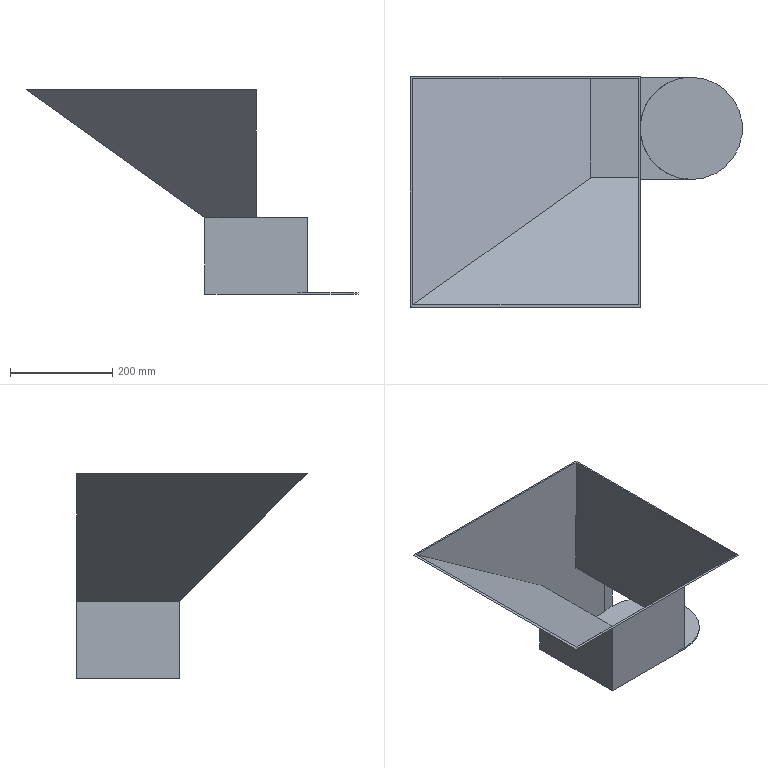Part | SolidWorks | features ICE 2, Blend 1, Extrusion 1, Shell 1 | 1 solid | 20 faces | box 650 x 450 x 400 mm | volume 1573727 mm3 | plane 18 | cylinder 2 | commonest cylinder face diameters 200 x2
STEP:
#1=CARTESIAN_POINT('',(100.,-100.,3.));
#2=VERTEX_POINT('',#1);
#3=CARTESIAN_POINT('',(75.69,-97.,3.));
#4=VERTEX_POINT('',#3);
#5=CARTESIAN_POINT('',(100.,0.,3.));
#6=DIRECTION('',(0.,0.,-1.));
#7=DIRECTION('',(-1.,0.,0.));
#8=AXIS2_PLACEMENT_3D('',#5,#6,#7);
#9=CIRCLE('',#8,100.);
#10=EDGE_CURVE('',#2,#4,#9,.T.);
#11=ORIENTED_EDGE('',*,*,#10,.T.);
#12=CARTESIAN_POINT('',(75.69,-97.,147.));
#13=VERTEX_POINT('',#12);
#14=CARTESIAN_POINT('',(75.69,-97.,-50.));
#15=DIRECTION('',(0.,0.,-1.));
#16=VECTOR('',#15,1000.);
#17=LINE('',#14,#16);
#18=EDGE_CURVE('',#13,#4,#17,.T.);
#19=ORIENTED_EDGE('',*,*,#18,.F.);
#20=CARTESIAN_POINT('',(75.69,97.,147.));
#21=VERTEX_POINT('',#20);
#22=CARTESIAN_POINT('',(100.,0.,147.));
#23=DIRECTION('',(0.,0.,1.));
#24=DIRECTION('',(-1.,0.,0.));
#25=AXIS2_PLACEMENT_3D('',#22,#23,#24);
#26=CIRCLE('',#25,100.);
#27=EDGE_CURVE('',#21,#13,#26,.T.);
#28=ORIENTED_EDGE('',*,*,#27,.F.);
#29=CARTESIAN_POINT('',(75.69,97.,3.));
#30=VERTEX_POINT('',#29);
#31=CARTESIAN_POINT('',(75.69,97.,75.));
#32=DIRECTION('',(0.,0.,-1.));
#33=VECTOR('',#32,1000.);
#34=LINE('',#31,#33);
#35=EDGE_CURVE('',#21,#30,#34,.T.);
#36=ORIENTED_EDGE('',*,*,#35,.T.);
#37=CARTESIAN_POINT('',(100.,100.,3.));
#38=VERTEX_POINT('',#37);
#39=CARTESIAN_POINT('',(100.,0.,3.));
#40=DIRECTION('',(0.,0.,-1.));
#41=DIRECTION('',(-1.,0.,0.));
#42=AXIS2_PLACEMENT_3D('',#39,#40,#41);
#43=CIRCLE('',#42,100.);
#44=EDGE_CURVE('',#30,#38,#43,.T.);
#45=ORIENTED_EDGE('',*,*,#44,.T.);
#46=CARTESIAN_POINT('',(100.,100.,150.));
#47=VERTEX_POINT('',#46);
#48=CARTESIAN_POINT('',(100.,100.,150.));
#49=DIRECTION('',(0.,0.,-1.));
#50=VECTOR('',#49,1000.);
#51=LINE('',#48,#50);
#52=EDGE_CURVE('',#47,#38,#51,.T.);
#53=ORIENTED_EDGE('',*,*,#52,.F.);
#54=CARTESIAN_POINT('',(0.,0.,150.));
#55=VERTEX_POINT('',#54);
#56=CARTESIAN_POINT('',(100.,0.,150.));
#57=DIRECTION('',(0.,0.,1.));
#58=DIRECTION('',(1.,0.,0.));
#59=AXIS2_PLACEMENT_3D('',#56,#57,#58);
#60=CIRCLE('',#59,100.);
#61=EDGE_CURVE('',#47,#55,#60,.T.);
#62=ORIENTED_EDGE('',*,*,#61,.T.);
#63=CARTESIAN_POINT('',(100.,-100.,150.));
#64=VERTEX_POINT('',#63);
#65=CARTESIAN_POINT('',(100.,0.,150.));
#66=DIRECTION('',(0.,0.,1.));
#67=DIRECTION('',(1.,0.,0.));
#68=AXIS2_PLACEMENT_3D('',#65,#66,#67);
#69=CIRCLE('',#68,100.);
#70=EDGE_CURVE('',#55,#64,#69,.T.);
#71=ORIENTED_EDGE('',*,*,#70,.T.);
#72=CARTESIAN_POINT('',(100.,-100.,150.));
#73=DIRECTION('',(0.,0.,-1.));
#74=VECTOR('',#73,1000.);
#75=LINE('',#72,#74);
#76=EDGE_CURVE('',#64,#2,#75,.T.);
#77=ORIENTED_EDGE('',*,*,#76,.T.);
#78=EDGE_LOOP('',(#11,#19,#28,#36,#45,#53,#62,#71,#77));
#79=FACE_OUTER_BOUND('',#78,.T.);
#80=CARTESIAN_POINT('',(100.,0.,-50.));
#81=DIRECTION('',(0.,0.,1.));
#82=DIRECTION('',(1.,0.,0.));
#83=AXIS2_PLACEMENT_3D('',#80,#81,#82);
#84=CYLINDRICAL_SURFACE('',#83,100.);
#85=ADVANCED_FACE('',(#79),#84,.F.);
#86=CARTESIAN_POINT('',(-97.,-97.,151.243));
#87=VERTEX_POINT('',#86);
#88=CARTESIAN_POINT('',(-97.,-97.,3.));
#89=VERTEX_POINT('',#88);
#90=CARTESIAN_POINT('',(-97.,-97.,150.));
#91=DIRECTION('',(0.,0.,-1.));
#92=VECTOR('',#91,1000.);
#93=LINE('',#90,#92);
#94=EDGE_CURVE('',#87,#89,#93,.T.);
#95=ORIENTED_EDGE('',*,*,#94,.T.);
#96=CARTESIAN_POINT('',(-97.,97.,3.));
#97=VERTEX_POINT('',#96);
#98=CARTESIAN_POINT('',(-97.,0.,3.));
#99=DIRECTION('',(0.,-1.,0.));
#100=VECTOR('',#99,1000.);
#101=LINE('',#98,#100);
#102=EDGE_CURVE('',#97,#89,#101,.T.);
#103=ORIENTED_EDGE('',*,*,#102,.F.);
#104=CARTESIAN_POINT('',(-97.,97.,151.544));
#105=VERTEX_POINT('',#104);
#106=CARTESIAN_POINT('',(-97.,97.,150.));
#107=DIRECTION('',(0.,0.,-1.));
#108=VECTOR('',#107,1000.);
#109=LINE('',#106,#108);
#110=EDGE_CURVE('',#105,#97,#109,.T.);
#111=ORIENTED_EDGE('',*,*,#110,.F.);
#112=CARTESIAN_POINT('',(-97.,-97.301,151.544));
#113=VERTEX_POINT('',#112);
#114=CARTESIAN_POINT('',(-97.,0.,151.544));
#115=DIRECTION('',(0.,-1.,0.));
#116=VECTOR('',#115,1000.);
#117=LINE('',#114,#116);
#118=EDGE_CURVE('',#105,#113,#117,.T.);
#119=ORIENTED_EDGE('',*,*,#118,.T.);
#120=CARTESIAN_POINT('',(-97.,27.121,27.121));
#121=DIRECTION('',(0.,-0.7071,0.7071));
#122=VECTOR('',#121,1000.);
#123=LINE('',#120,#122);
#124=EDGE_CURVE('',#87,#113,#123,.T.);
#125=ORIENTED_EDGE('',*,*,#124,.F.);
#126=EDGE_LOOP('',(#95,#103,#111,#119,#125));
#127=FACE_OUTER_BOUND('',#126,.T.);
#128=CARTESIAN_POINT('',(-97.,100.,150.));
#129=DIRECTION('',(1.,0.,0.));
#130=DIRECTION('',(0.,1.,0.));
#131=AXIS2_PLACEMENT_3D('',#128,#129,#130);
#132=PLANE('',#131);
#133=ADVANCED_FACE('',(#127),#132,.T.);
#134=ORIENTED_EDGE('',*,*,#18,.T.);
#135=CARTESIAN_POINT('',(0.,-97.,3.));
#136=DIRECTION('',(1.,0.,0.));
#137=VECTOR('',#136,1000.);
#138=LINE('',#135,#137);
#139=EDGE_CURVE('',#89,#4,#138,.T.);
#140=ORIENTED_EDGE('',*,*,#139,.F.);
#141=ORIENTED_EDGE('',*,*,#94,.F.);
#142=CARTESIAN_POINT('',(-3.,-97.,151.243));
#143=VERTEX_POINT('',#142);
#144=CARTESIAN_POINT('',(0.,-97.,151.243));
#145=DIRECTION('',(1.,0.,0.));
#146=VECTOR('',#145,1000.);
#147=LINE('',#144,#146);
#148=EDGE_CURVE('',#87,#143,#147,.T.);
#149=ORIENTED_EDGE('',*,*,#148,.T.);
#150=CARTESIAN_POINT('',(-3.,-97.,147.));
#151=VERTEX_POINT('',#150);
#152=CARTESIAN_POINT('',(-3.,-97.,150.));
#153=DIRECTION('',(0.,0.,-1.));
#154=VECTOR('',#153,1000.);
#155=LINE('',#152,#154);
#156=EDGE_CURVE('',#143,#151,#155,.T.);
#157=ORIENTED_EDGE('',*,*,#156,.T.);
#158=CARTESIAN_POINT('',(0.,-97.,147.));
#159=DIRECTION('',(1.,0.,0.));
#160=VECTOR('',#159,1000.);
#161=LINE('',#158,#160);
#162=EDGE_CURVE('',#151,#13,#161,.T.);
#163=ORIENTED_EDGE('',*,*,#162,.T.);
#164=EDGE_LOOP('',(#134,#140,#141,#149,#157,#163));
#165=FACE_OUTER_BOUND('',#164,.T.);
#166=CARTESIAN_POINT('',(100.,-97.,150.));
#167=DIRECTION('',(0.,1.,0.));
#168=DIRECTION('',(-1.,0.,0.));
#169=AXIS2_PLACEMENT_3D('',#166,#167,#168);
#170=PLANE('',#169);
#171=ADVANCED_FACE('',(#165),#170,.T.);
#172=ORIENTED_EDGE('',*,*,#110,.T.);
#173=CARTESIAN_POINT('',(0.,97.,3.));
#174=DIRECTION('',(-1.,0.,0.));
#175=VECTOR('',#174,1000.);
#176=LINE('',#173,#175);
#177=EDGE_CURVE('',#30,#97,#176,.T.);
#178=ORIENTED_EDGE('',*,*,#177,.F.);
#179=ORIENTED_EDGE('',*,*,#35,.F.);
#180=CARTESIAN_POINT('',(-3.,97.,147.));
#181=VERTEX_POINT('',#180);
#182=CARTESIAN_POINT('',(0.,97.,147.));
#183=DIRECTION('',(-1.,0.,0.));
#184=VECTOR('',#183,1000.);
#185=LINE('',#182,#184);
#186=EDGE_CURVE('',#21,#181,#185,.T.);
#187=ORIENTED_EDGE('',*,*,#186,.T.);
#188=CARTESIAN_POINT('',(-3.,97.,400.));
#189=VERTEX_POINT('',#188);
#190=CARTESIAN_POINT('',(-3.,97.,0.));
#191=DIRECTION('',(0.,0.,-1.));
#192=VECTOR('',#191,1000.);
#193=LINE('',#190,#192);
#194=EDGE_CURVE('',#189,#181,#193,.T.);
#195=ORIENTED_EDGE('',*,*,#194,.F.);
#196=CARTESIAN_POINT('',(-444.839,97.,400.));
#197=VERTEX_POINT('',#196);
#198=CARTESIAN_POINT('',(0.,97.,400.));
#199=DIRECTION('',(-1.,0.,0.));
#200=VECTOR('',#199,1000.);
#201=LINE('',#198,#200);
#202=EDGE_CURVE('',#189,#197,#201,.T.);
#203=ORIENTED_EDGE('',*,*,#202,.T.);
#204=CARTESIAN_POINT('',(34.176,97.,57.847));
#205=DIRECTION('',(0.8137,0.,-0.5812));
#206=VECTOR('',#205,1000.);
#207=LINE('',#204,#206);
#208=EDGE_CURVE('',#197,#105,#207,.T.);
#209=ORIENTED_EDGE('',*,*,#208,.T.);
#210=EDGE_LOOP('',(#172,#178,#179,#187,#195,#203,#209));
#211=FACE_OUTER_BOUND('',#210,.T.);
#212=CARTESIAN_POINT('',(100.,97.,150.));
#213=DIRECTION('',(0.,-1.,0.));
#214=DIRECTION('',(1.,0.,0.));
#215=AXIS2_PLACEMENT_3D('',#212,#213,#214);
#216=PLANE('',#215);
#217=ADVANCED_FACE('',(#211),#216,.T.);
#218=CARTESIAN_POINT('',(100.,100.,0.));
#219=VERTEX_POINT('',#218);
#220=CARTESIAN_POINT('',(-100.,100.,0.));
#221=VERTEX_POINT('',#220);
#222=CARTESIAN_POINT('',(100.,100.,0.));
#223=DIRECTION('',(-1.,0.,0.));
#224=VECTOR('',#223,1000.);
#225=LINE('',#222,#224);
#226=EDGE_CURVE('',#219,#221,#225,.T.);
#227=ORIENTED_EDGE('',*,*,#226,.F.);
#228=CARTESIAN_POINT('',(100.,-100.,0.));
#229=VERTEX_POINT('',#228);
#230=CARTESIAN_POINT('',(100.,0.,0.));
#231=DIRECTION('',(0.,0.,-1.));
#232=DIRECTION('',(-1.,0.,0.));
#233=AXIS2_PLACEMENT_3D('',#230,#231,#232);
#234=CIRCLE('',#233,100.);
#235=EDGE_CURVE('',#219,#229,#234,.T.);
#236=ORIENTED_EDGE('',*,*,#235,.T.);
#237=CARTESIAN_POINT('',(-100.,-100.,0.));
#238=VERTEX_POINT('',#237);
#239=CARTESIAN_POINT('',(100.,-100.,0.));
#240=DIRECTION('',(1.,0.,0.));
#241=VECTOR('',#240,1000.);
#242=LINE('',#239,#241);
#243=EDGE_CURVE('',#238,#229,#242,.T.);
#244=ORIENTED_EDGE('',*,*,#243,.F.);
#245=CARTESIAN_POINT('',(-100.,100.,0.));
#246=DIRECTION('',(0.,-1.,0.));
#247=VECTOR('',#246,1000.);
#248=LINE('',#245,#247);
#249=EDGE_CURVE('',#221,#238,#248,.T.);
#250=ORIENTED_EDGE('',*,*,#249,.F.);
#251=EDGE_LOOP('',(#227,#236,#244,#250));
#252=FACE_OUTER_BOUND('',#251,.T.);
#253=CARTESIAN_POINT('',(0.,0.,0.));
#254=DIRECTION('',(0.,0.,-1.));
#255=DIRECTION('',(-1.,0.,0.));
#256=AXIS2_PLACEMENT_3D('',#253,#254,#255);
#257=PLANE('',#256);
#258=ADVANCED_FACE('',(#252),#257,.T.);
#259=CARTESIAN_POINT('',(0.,-350.,400.));
#260=VERTEX_POINT('',#259);
#261=CARTESIAN_POINT('',(0.,100.,400.));
#262=VERTEX_POINT('',#261);
#263=CARTESIAN_POINT('',(0.,100.,400.));
#264=DIRECTION('',(0.,1.,0.));
#265=VECTOR('',#264,1000.);
#266=LINE('',#263,#265);
#267=EDGE_CURVE('',#260,#262,#266,.T.);
#268=ORIENTED_EDGE('',*,*,#267,.T.);
#269=CARTESIAN_POINT('',(-450.,100.,400.));
#270=VERTEX_POINT('',#269);
#271=CARTESIAN_POINT('',(0.,100.,400.));
#272=DIRECTION('',(-1.,0.,0.));
#273=VECTOR('',#272,1000.);
#274=LINE('',#271,#273);
#275=EDGE_CURVE('',#262,#270,#274,.T.);
#276=ORIENTED_EDGE('',*,*,#275,.T.);
#277=CARTESIAN_POINT('',(-450.,-350.,400.));
#278=VERTEX_POINT('',#277);
#279=CARTESIAN_POINT('',(-450.,100.,400.));
#280=DIRECTION('',(0.,-1.,0.));
#281=VECTOR('',#280,1000.);
#282=LINE('',#279,#281);
#283=EDGE_CURVE('',#270,#278,#282,.T.);
#284=ORIENTED_EDGE('',*,*,#283,.T.);
#285=CARTESIAN_POINT('',(0.,-350.,400.));
#286=DIRECTION('',(1.,0.,0.));
#287=VECTOR('',#286,1000.);
#288=LINE('',#285,#287);
#289=EDGE_CURVE('',#278,#260,#288,.T.);
#290=ORIENTED_EDGE('',*,*,#289,.T.);
#291=EDGE_LOOP('',(#268,#276,#284,#290));
#292=FACE_OUTER_BOUND('',#291,.T.);
#293=CARTESIAN_POINT('',(-3.,-345.757,400.));
#294=VERTEX_POINT('',#293);
#295=CARTESIAN_POINT('',(-3.,0.,400.));
#296=DIRECTION('',(0.,1.,0.));
#297=VECTOR('',#296,1000.);
#298=LINE('',#295,#297);
#299=EDGE_CURVE('',#294,#189,#298,.T.);
#300=ORIENTED_EDGE('',*,*,#299,.F.);
#301=CARTESIAN_POINT('',(-444.839,-345.757,400.));
#302=VERTEX_POINT('',#301);
#303=CARTESIAN_POINT('',(0.,-345.757,400.));
#304=DIRECTION('',(1.,0.,0.));
#305=VECTOR('',#304,1000.);
#306=LINE('',#303,#305);
#307=EDGE_CURVE('',#302,#294,#306,.T.);
#308=ORIENTED_EDGE('',*,*,#307,.F.);
#309=CARTESIAN_POINT('',(-444.839,0.,400.));
#310=DIRECTION('',(0.,-1.,0.));
#311=VECTOR('',#310,1000.);
#312=LINE('',#309,#311);
#313=EDGE_CURVE('',#197,#302,#312,.T.);
#314=ORIENTED_EDGE('',*,*,#313,.F.);
#315=ORIENTED_EDGE('',*,*,#202,.F.);
#316=EDGE_LOOP('',(#300,#308,#314,#315));
#317=FACE_BOUND('',#316,.T.);
#318=CARTESIAN_POINT('',(0.,0.,400.));
#319=DIRECTION('',(0.,0.,-1.));
#320=DIRECTION('',(-1.,0.,0.));
#321=AXIS2_PLACEMENT_3D('',#318,#319,#320);
#322=PLANE('',#321);
#323=ADVANCED_FACE('',(#292,#317),#322,.F.);
#324=CARTESIAN_POINT('',(0.,100.,150.));
#325=VERTEX_POINT('',#324);
#326=CARTESIAN_POINT('',(0.,100.,150.));
#327=DIRECTION('',(0.,1.,0.));
#328=VECTOR('',#327,1000.);
#329=LINE('',#326,#328);
#330=EDGE_CURVE('',#55,#325,#329,.T.);
#331=ORIENTED_EDGE('',*,*,#330,.F.);
#332=ORIENTED_EDGE('',*,*,#61,.F.);
#333=CARTESIAN_POINT('',(100.,100.,150.));
#334=DIRECTION('',(-1.,0.,0.));
#335=VECTOR('',#334,1000.);
#336=LINE('',#333,#335);
#337=EDGE_CURVE('',#47,#325,#336,.T.);
#338=ORIENTED_EDGE('',*,*,#337,.T.);
#339=EDGE_LOOP('',(#331,#332,#338));
#340=FACE_OUTER_BOUND('',#339,.T.);
#341=CARTESIAN_POINT('',(0.,0.,150.));
#342=DIRECTION('',(0.,0.,-1.));
#343=DIRECTION('',(-1.,0.,0.));
#344=AXIS2_PLACEMENT_3D('',#341,#342,#343);
#345=PLANE('',#344);
#346=ADVANCED_FACE('',(#340),#345,.F.);
#347=ORIENTED_EDGE('',*,*,#249,.T.);
#348=CARTESIAN_POINT('',(-100.,-100.,150.));
#349=VERTEX_POINT('',#348);
#350=CARTESIAN_POINT('',(-100.,-100.,150.));
#351=DIRECTION('',(0.,0.,-1.));
#352=VECTOR('',#351,1000.);
#353=LINE('',#350,#352);
#354=EDGE_CURVE('',#349,#238,#353,.T.);
#355=ORIENTED_EDGE('',*,*,#354,.F.);
#356=CARTESIAN_POINT('',(-100.,100.,150.));
#357=VERTEX_POINT('',#356);
#358=CARTESIAN_POINT('',(-100.,0.,150.));
#359=DIRECTION('',(0.,-1.,0.));
#360=VECTOR('',#359,1000.);
#361=LINE('',#358,#360);
#362=EDGE_CURVE('',#357,#349,#361,.T.);
#363=ORIENTED_EDGE('',*,*,#362,.F.);
#364=CARTESIAN_POINT('',(-100.,100.,150.));
#365=DIRECTION('',(0.,0.,-1.));
#366=VECTOR('',#365,1000.);
#367=LINE('',#364,#366);
#368=EDGE_CURVE('',#357,#221,#367,.T.);
#369=ORIENTED_EDGE('',*,*,#368,.T.);
#370=EDGE_LOOP('',(#347,#355,#363,#369));
#371=FACE_OUTER_BOUND('',#370,.T.);
#372=CARTESIAN_POINT('',(-100.,100.,150.));
#373=DIRECTION('',(1.,0.,0.));
#374=DIRECTION('',(0.,1.,0.));
#375=AXIS2_PLACEMENT_3D('',#372,#373,#374);
#376=PLANE('',#375);
#377=ADVANCED_FACE('',(#371),#376,.F.);
#378=ORIENTED_EDGE('',*,*,#243,.T.);
#379=CARTESIAN_POINT('',(100.,-100.,3.));
#380=DIRECTION('',(0.,0.,-1.));
#381=VECTOR('',#380,1000.);
#382=LINE('',#379,#381);
#383=EDGE_CURVE('',#2,#229,#382,.T.);
#384=ORIENTED_EDGE('',*,*,#383,.F.);
#385=ORIENTED_EDGE('',*,*,#76,.F.);
#386=CARTESIAN_POINT('',(0.,-100.,150.));
#387=VERTEX_POINT('',#386);
#388=CARTESIAN_POINT('',(100.,-100.,150.));
#389=DIRECTION('',(1.,0.,0.));
#390=VECTOR('',#389,1000.);
#391=LINE('',#388,#390);
#392=EDGE_CURVE('',#387,#64,#391,.T.);
#393=ORIENTED_EDGE('',*,*,#392,.F.);
#394=CARTESIAN_POINT('',(0.,-100.,150.));
#395=DIRECTION('',(1.,0.,0.));
#396=VECTOR('',#395,1000.);
#397=LINE('',#394,#396);
#398=EDGE_CURVE('',#349,#387,#397,.T.);
#399=ORIENTED_EDGE('',*,*,#398,.F.);
#400=ORIENTED_EDGE('',*,*,#354,.T.);
#401=EDGE_LOOP('',(#378,#384,#385,#393,#399,#400));
#402=FACE_OUTER_BOUND('',#401,.T.);
#403=CARTESIAN_POINT('',(100.,-100.,150.));
#404=DIRECTION('',(0.,1.,0.));
#405=DIRECTION('',(-1.,0.,0.));
#406=AXIS2_PLACEMENT_3D('',#403,#404,#405);
#407=PLANE('',#406);
#408=ADVANCED_FACE('',(#402),#407,.F.);
#409=ORIENTED_EDGE('',*,*,#226,.T.);
#410=ORIENTED_EDGE('',*,*,#368,.F.);
#411=CARTESIAN_POINT('',(-450.,100.,400.));
#412=DIRECTION('',(0.8137,0.,-0.5812));
#413=VECTOR('',#412,1000.);
#414=LINE('',#411,#413);
#415=EDGE_CURVE('',#270,#357,#414,.T.);
#416=ORIENTED_EDGE('',*,*,#415,.F.);
#417=ORIENTED_EDGE('',*,*,#275,.F.);
#418=CARTESIAN_POINT('',(0.,100.,400.));
#419=DIRECTION('',(0.,0.,-1.));
#420=VECTOR('',#419,1000.);
#421=LINE('',#418,#420);
#422=EDGE_CURVE('',#262,#325,#421,.T.);
#423=ORIENTED_EDGE('',*,*,#422,.T.);
#424=ORIENTED_EDGE('',*,*,#337,.F.);
#425=ORIENTED_EDGE('',*,*,#52,.T.);
#426=CARTESIAN_POINT('',(100.,100.,3.));
#427=DIRECTION('',(0.,0.,-1.));
#428=VECTOR('',#427,1000.);
#429=LINE('',#426,#428);
#430=EDGE_CURVE('',#38,#219,#429,.T.);
#431=ORIENTED_EDGE('',*,*,#430,.T.);
#432=EDGE_LOOP('',(#409,#410,#416,#417,#423,#424,#425,#431));
#433=FACE_OUTER_BOUND('',#432,.T.);
#434=CARTESIAN_POINT('',(100.,100.,150.));
#435=DIRECTION('',(0.,-1.,0.));
#436=DIRECTION('',(1.,0.,0.));
#437=AXIS2_PLACEMENT_3D('',#434,#435,#436);
#438=PLANE('',#437);
#439=ADVANCED_FACE('',(#433),#438,.F.);
#440=ORIENTED_EDGE('',*,*,#392,.T.);
#441=ORIENTED_EDGE('',*,*,#70,.F.);
#442=CARTESIAN_POINT('',(0.,100.,150.));
#443=DIRECTION('',(0.,1.,0.));
#444=VECTOR('',#443,1000.);
#445=LINE('',#442,#444);
#446=EDGE_CURVE('',#387,#55,#445,.T.);
#447=ORIENTED_EDGE('',*,*,#446,.F.);
#448=EDGE_LOOP('',(#440,#441,#447));
#449=FACE_OUTER_BOUND('',#448,.T.);
#450=CARTESIAN_POINT('',(0.,0.,150.));
#451=DIRECTION('',(0.,0.,-1.));
#452=DIRECTION('',(-1.,0.,0.));
#453=AXIS2_PLACEMENT_3D('',#450,#451,#452);
#454=PLANE('',#453);
#455=ADVANCED_FACE('',(#449),#454,.F.);
#456=CARTESIAN_POINT('',(0.,-350.,400.));
#457=DIRECTION('',(0.,0.7071,-0.7071));
#458=VECTOR('',#457,1000.);
#459=LINE('',#456,#458);
#460=EDGE_CURVE('',#260,#387,#459,.T.);
#461=ORIENTED_EDGE('',*,*,#460,.T.);
#462=ORIENTED_EDGE('',*,*,#446,.T.);
#463=ORIENTED_EDGE('',*,*,#330,.T.);
#464=ORIENTED_EDGE('',*,*,#422,.F.);
#465=ORIENTED_EDGE('',*,*,#267,.F.);
#466=EDGE_LOOP('',(#461,#462,#463,#464,#465));
#467=FACE_OUTER_BOUND('',#466,.T.);
#468=CARTESIAN_POINT('',(0.,0.,0.));
#469=DIRECTION('',(1.,0.,0.));
#470=DIRECTION('',(0.,0.,-1.));
#471=AXIS2_PLACEMENT_3D('',#468,#469,#470);
#472=PLANE('',#471);
#473=ADVANCED_FACE('',(#467),#472,.T.);
#474=CARTESIAN_POINT('',(-450.,-350.,400.));
#475=DIRECTION('',(0.7035,0.5025,-0.5025));
#476=VECTOR('',#475,1000.);
#477=LINE('',#474,#476);
#478=EDGE_CURVE('',#278,#349,#477,.T.);
#479=ORIENTED_EDGE('',*,*,#478,.T.);
#480=ORIENTED_EDGE('',*,*,#398,.T.);
#481=ORIENTED_EDGE('',*,*,#460,.F.);
#482=ORIENTED_EDGE('',*,*,#289,.F.);
#483=EDGE_LOOP('',(#479,#480,#481,#482));
#484=FACE_OUTER_BOUND('',#483,.T.);
#485=CARTESIAN_POINT('',(0.,25.,25.));
#486=DIRECTION('',(0.,-0.7071,-0.7071));
#487=DIRECTION('',(0.,0.7071,-0.7071));
#488=AXIS2_PLACEMENT_3D('',#485,#486,#487);
#489=PLANE('',#488);
#490=ADVANCED_FACE('',(#484),#489,.T.);
#491=ORIENTED_EDGE('',*,*,#415,.T.);
#492=ORIENTED_EDGE('',*,*,#362,.T.);
#493=ORIENTED_EDGE('',*,*,#478,.F.);
#494=ORIENTED_EDGE('',*,*,#283,.F.);
#495=EDGE_LOOP('',(#491,#492,#493,#494));
#496=FACE_OUTER_BOUND('',#495,.T.);
#497=CARTESIAN_POINT('',(37.162,0.,52.027));
#498=DIRECTION('',(-0.5812,0.,-0.8137));
#499=DIRECTION('',(-0.8137,0.,0.5812));
#500=AXIS2_PLACEMENT_3D('',#497,#498,#499);
#501=PLANE('',#500);
#502=ADVANCED_FACE('',(#496),#501,.T.);
#503=ORIENTED_EDGE('',*,*,#162,.F.);
#504=CARTESIAN_POINT('',(-3.,0.,147.));
#505=DIRECTION('',(0.,1.,0.));
#506=VECTOR('',#505,1000.);
#507=LINE('',#504,#506);
#508=EDGE_CURVE('',#151,#181,#507,.T.);
#509=ORIENTED_EDGE('',*,*,#508,.T.);
#510=ORIENTED_EDGE('',*,*,#186,.F.);
#511=ORIENTED_EDGE('',*,*,#27,.T.);
#512=EDGE_LOOP('',(#503,#509,#510,#511));
#513=FACE_OUTER_BOUND('',#512,.T.);
#514=CARTESIAN_POINT('',(0.,0.,147.));
#515=DIRECTION('',(0.,0.,-1.));
#516=DIRECTION('',(-1.,0.,0.));
#517=AXIS2_PLACEMENT_3D('',#514,#515,#516);
#518=PLANE('',#517);
#519=ADVANCED_FACE('',(#513),#518,.T.);
#520=CARTESIAN_POINT('',(-3.,27.121,27.121));
#521=DIRECTION('',(0.,0.7071,-0.7071));
#522=VECTOR('',#521,1000.);
#523=LINE('',#520,#522);
#524=EDGE_CURVE('',#294,#143,#523,.T.);
#525=ORIENTED_EDGE('',*,*,#524,.F.);
#526=ORIENTED_EDGE('',*,*,#299,.T.);
#527=ORIENTED_EDGE('',*,*,#194,.T.);
#528=ORIENTED_EDGE('',*,*,#508,.F.);
#529=ORIENTED_EDGE('',*,*,#156,.F.);
#530=EDGE_LOOP('',(#525,#526,#527,#528,#529));
#531=FACE_OUTER_BOUND('',#530,.T.);
#532=CARTESIAN_POINT('',(-3.,0.,0.));
#533=DIRECTION('',(1.,0.,0.));
#534=DIRECTION('',(0.,0.,-1.));
#535=AXIS2_PLACEMENT_3D('',#532,#533,#534);
#536=PLANE('',#535);
#537=ADVANCED_FACE('',(#531),#536,.F.);
#538=CARTESIAN_POINT('',(38.986,-0.1686,54.411));
#539=DIRECTION('',(0.7035,0.5025,-0.5025));
#540=VECTOR('',#539,1000.);
#541=LINE('',#538,#540);
#542=EDGE_CURVE('',#302,#113,#541,.T.);
#543=ORIENTED_EDGE('',*,*,#542,.F.);
#544=ORIENTED_EDGE('',*,*,#307,.T.);
#545=ORIENTED_EDGE('',*,*,#524,.T.);
#546=ORIENTED_EDGE('',*,*,#148,.F.);
#547=ORIENTED_EDGE('',*,*,#124,.T.);
#548=EDGE_LOOP('',(#543,#544,#545,#546,#547));
#549=FACE_OUTER_BOUND('',#548,.T.);
#550=CARTESIAN_POINT('',(0.,27.121,27.121));
#551=DIRECTION('',(0.,-0.7071,-0.7071));
#552=DIRECTION('',(0.,0.7071,-0.7071));
#553=AXIS2_PLACEMENT_3D('',#550,#551,#552);
#554=PLANE('',#553);
#555=ADVANCED_FACE('',(#549),#554,.F.);
#556=ORIENTED_EDGE('',*,*,#208,.F.);
#557=ORIENTED_EDGE('',*,*,#313,.T.);
#558=ORIENTED_EDGE('',*,*,#542,.T.);
#559=ORIENTED_EDGE('',*,*,#118,.F.);
#560=EDGE_LOOP('',(#556,#557,#558,#559));
#561=FACE_OUTER_BOUND('',#560,.T.);
#562=CARTESIAN_POINT('',(38.906,0.,54.468));
#563=DIRECTION('',(-0.5812,0.,-0.8137));
#564=DIRECTION('',(-0.8137,0.,0.5812));
#565=AXIS2_PLACEMENT_3D('',#562,#563,#564);
#566=PLANE('',#565);
#567=ADVANCED_FACE('',(#561),#566,.F.);
#568=CARTESIAN_POINT('',(100.,0.,3.));
#569=DIRECTION('',(0.,0.,-1.));
#570=DIRECTION('',(-1.,0.,0.));
#571=AXIS2_PLACEMENT_3D('',#568,#569,#570);
#572=CIRCLE('',#571,100.);
#573=EDGE_CURVE('',#38,#2,#572,.T.);
#574=ORIENTED_EDGE('',*,*,#573,.T.);
#575=ORIENTED_EDGE('',*,*,#383,.T.);
#576=ORIENTED_EDGE('',*,*,#235,.F.);
#577=ORIENTED_EDGE('',*,*,#430,.F.);
#578=EDGE_LOOP('',(#574,#575,#576,#577));
#579=FACE_OUTER_BOUND('',#578,.T.);
#580=CARTESIAN_POINT('',(100.,0.,3.));
#581=DIRECTION('',(0.,0.,-1.));
#582=DIRECTION('',(-1.,0.,0.));
#583=AXIS2_PLACEMENT_3D('',#580,#581,#582);
#584=CYLINDRICAL_SURFACE('',#583,100.);
#585=ADVANCED_FACE('',(#579),#584,.T.);
#586=ORIENTED_EDGE('',*,*,#44,.F.);
#587=ORIENTED_EDGE('',*,*,#177,.T.);
#588=ORIENTED_EDGE('',*,*,#102,.T.);
#589=ORIENTED_EDGE('',*,*,#139,.T.);
#590=ORIENTED_EDGE('',*,*,#10,.F.);
#591=ORIENTED_EDGE('',*,*,#573,.F.);
#592=EDGE_LOOP('',(#586,#587,#588,#589,#590,#591));
#593=FACE_OUTER_BOUND('',#592,.T.);
#594=CARTESIAN_POINT('',(0.,0.,3.));
#595=DIRECTION('',(0.,0.,-1.));
#596=DIRECTION('',(-1.,0.,0.));
#597=AXIS2_PLACEMENT_3D('',#594,#595,#596);
#598=PLANE('',#597);
#599=ADVANCED_FACE('',(#593),#598,.F.);
#600=CLOSED_SHELL('',(#85,#133,#171,#217,#258,#323,#346,#377,#408,#439,#455,#473,#490,#502,#519,#537,#555,#567,#585,#599));
#601=MANIFOLD_SOLID_BREP('',#600);
#602=CARTESIAN_POINT('',(0.,0.,0.));
#603=DIRECTION('',(0.,0.,1.));
#604=DIRECTION('',(1.,0.,0.));
#605=AXIS2_PLACEMENT_3D('',#602,#603,#604);
#606=(LENGTH_UNIT()NAMED_UNIT(*)SI_UNIT(.MILLI.,.METRE.));
#607=UNCERTAINTY_MEASURE_WITH_UNIT(LENGTH_MEASURE(0.00001),#606,'','');
#608=(NAMED_UNIT(*)PLANE_ANGLE_UNIT()SI_UNIT($,.RADIAN.));
#609=(NAMED_UNIT(*)SI_UNIT($,.STERADIAN.)SOLID_ANGLE_UNIT());
#610=(GEOMETRIC_REPRESENTATION_CONTEXT(3)GLOBAL_UNCERTAINTY_ASSIGNED_CONTEXT((#607))GLOBAL_UNIT_ASSIGNED_CONTEXT((#606,#608,#609))REPRESENTATION_CONTEXT('',''));
#611=ADVANCED_BREP_SHAPE_REPRESENTATION('',(#601,#605),#610);